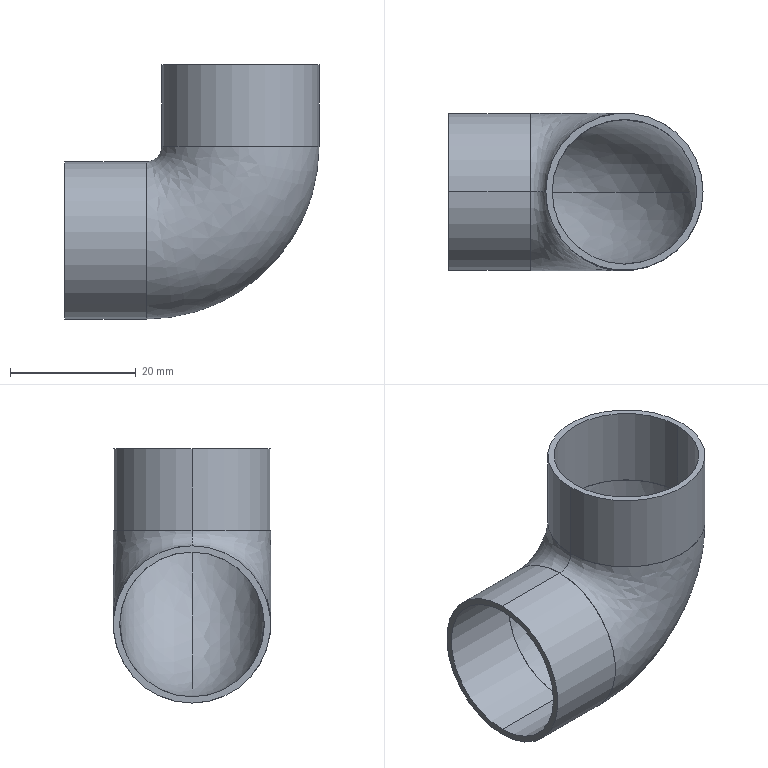Part | STEP file | one-inch elbow_default_machined_ | 3 solids | 18 faces | box 40.4 x 25 x 40.4 mm | volume 3722 mm3 | cylinder 8 | plane 6 | spline 4 | commonest cylinder face diameters 23 x4 25 x4